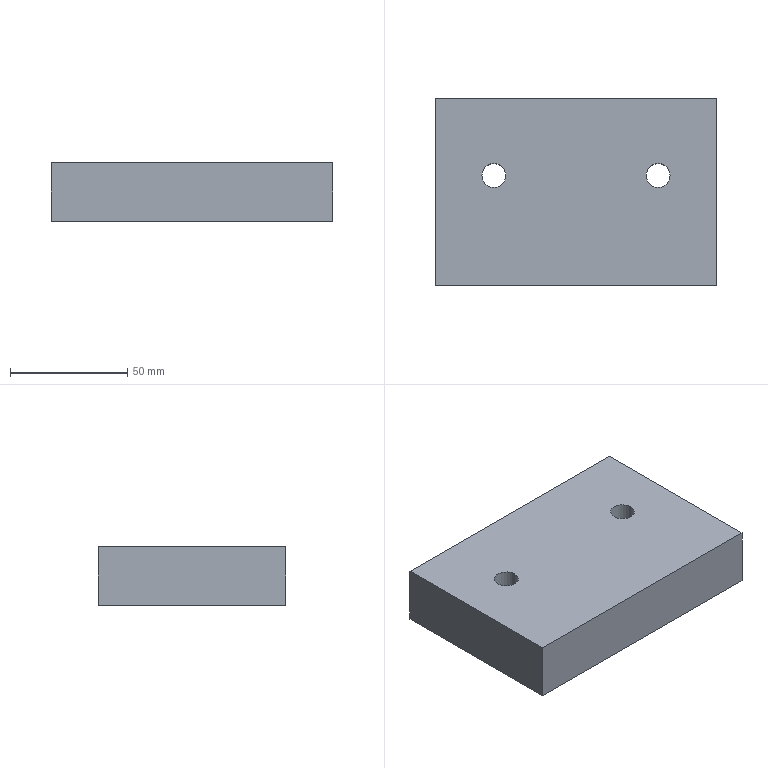Part | SolidWorks | features Extrusion 1, HoleWzd 1 | 1 solid | 10 faces | box 120 x 80 x 25 mm | volume 235914 mm3 | plane 6 | cylinder 4 | commonest cylinder face diameters 10.2 x4
STEP:
#1=CARTESIAN_POINT('',(-29.9,7.,0.));
#2=VERTEX_POINT('',#1);
#3=CARTESIAN_POINT('',(-40.1,7.,0.));
#4=VERTEX_POINT('',#3);
#5=CARTESIAN_POINT('',(-35.,7.,0.));
#6=DIRECTION('',(0.,0.,-1.));
#7=DIRECTION('',(-1.,0.,0.));
#8=AXIS2_PLACEMENT_3D('',#5,#6,#7);
#9=CIRCLE('',#8,5.1);
#10=EDGE_CURVE('',#2,#4,#9,.T.);
#11=ORIENTED_EDGE('',*,*,#10,.T.);
#12=CARTESIAN_POINT('',(-40.1,7.,25.));
#13=VERTEX_POINT('',#12);
#14=CARTESIAN_POINT('',(-40.1,7.,25.));
#15=DIRECTION('',(0.,0.,1.));
#16=VECTOR('',#15,1000.);
#17=LINE('',#14,#16);
#18=EDGE_CURVE('',#4,#13,#17,.T.);
#19=ORIENTED_EDGE('',*,*,#18,.T.);
#20=CARTESIAN_POINT('',(-29.9,7.,25.));
#21=VERTEX_POINT('',#20);
#22=CARTESIAN_POINT('',(-35.,7.,25.));
#23=DIRECTION('',(0.,0.,1.));
#24=DIRECTION('',(1.,0.,0.));
#25=AXIS2_PLACEMENT_3D('',#22,#23,#24);
#26=CIRCLE('',#25,5.1);
#27=EDGE_CURVE('',#13,#21,#26,.T.);
#28=ORIENTED_EDGE('',*,*,#27,.T.);
#29=CARTESIAN_POINT('',(-29.9,7.,25.));
#30=DIRECTION('',(0.,0.,1.));
#31=VECTOR('',#30,1000.);
#32=LINE('',#29,#31);
#33=EDGE_CURVE('',#2,#21,#32,.T.);
#34=ORIENTED_EDGE('',*,*,#33,.F.);
#35=EDGE_LOOP('',(#11,#19,#28,#34));
#36=FACE_OUTER_BOUND('',#35,.T.);
#37=CARTESIAN_POINT('',(-35.,7.,25.));
#38=DIRECTION('',(0.,0.,1.));
#39=DIRECTION('',(1.,0.,0.));
#40=AXIS2_PLACEMENT_3D('',#37,#38,#39);
#41=CYLINDRICAL_SURFACE('',#40,5.1);
#42=ADVANCED_FACE('',(#36),#41,.F.);
#43=CARTESIAN_POINT('',(40.1,7.,0.));
#44=VERTEX_POINT('',#43);
#45=CARTESIAN_POINT('',(29.9,7.,0.));
#46=VERTEX_POINT('',#45);
#47=CARTESIAN_POINT('',(35.,7.,0.));
#48=DIRECTION('',(0.,0.,-1.));
#49=DIRECTION('',(-1.,0.,0.));
#50=AXIS2_PLACEMENT_3D('',#47,#48,#49);
#51=CIRCLE('',#50,5.1);
#52=EDGE_CURVE('',#44,#46,#51,.T.);
#53=ORIENTED_EDGE('',*,*,#52,.T.);
#54=CARTESIAN_POINT('',(29.9,7.,25.));
#55=VERTEX_POINT('',#54);
#56=CARTESIAN_POINT('',(29.9,7.,25.));
#57=DIRECTION('',(0.,0.,1.));
#58=VECTOR('',#57,1000.);
#59=LINE('',#56,#58);
#60=EDGE_CURVE('',#46,#55,#59,.T.);
#61=ORIENTED_EDGE('',*,*,#60,.T.);
#62=CARTESIAN_POINT('',(40.1,7.,25.));
#63=VERTEX_POINT('',#62);
#64=CARTESIAN_POINT('',(35.,7.,25.));
#65=DIRECTION('',(0.,0.,1.));
#66=DIRECTION('',(1.,0.,0.));
#67=AXIS2_PLACEMENT_3D('',#64,#65,#66);
#68=CIRCLE('',#67,5.1);
#69=EDGE_CURVE('',#55,#63,#68,.T.);
#70=ORIENTED_EDGE('',*,*,#69,.T.);
#71=CARTESIAN_POINT('',(40.1,7.,25.));
#72=DIRECTION('',(0.,0.,1.));
#73=VECTOR('',#72,1000.);
#74=LINE('',#71,#73);
#75=EDGE_CURVE('',#44,#63,#74,.T.);
#76=ORIENTED_EDGE('',*,*,#75,.F.);
#77=EDGE_LOOP('',(#53,#61,#70,#76));
#78=FACE_OUTER_BOUND('',#77,.T.);
#79=CARTESIAN_POINT('',(35.,7.,25.));
#80=DIRECTION('',(0.,0.,1.));
#81=DIRECTION('',(1.,0.,0.));
#82=AXIS2_PLACEMENT_3D('',#79,#80,#81);
#83=CYLINDRICAL_SURFACE('',#82,5.1);
#84=ADVANCED_FACE('',(#78),#83,.F.);
#85=CARTESIAN_POINT('',(-60.,40.,0.));
#86=VERTEX_POINT('',#85);
#87=CARTESIAN_POINT('',(-60.,-40.,0.));
#88=VERTEX_POINT('',#87);
#89=CARTESIAN_POINT('',(-60.,40.,0.));
#90=DIRECTION('',(0.,-1.,0.));
#91=VECTOR('',#90,1000.);
#92=LINE('',#89,#91);
#93=EDGE_CURVE('',#86,#88,#92,.T.);
#94=ORIENTED_EDGE('',*,*,#93,.T.);
#95=CARTESIAN_POINT('',(-60.,-40.,25.));
#96=VERTEX_POINT('',#95);
#97=CARTESIAN_POINT('',(-60.,-40.,25.));
#98=DIRECTION('',(0.,0.,-1.));
#99=VECTOR('',#98,1000.);
#100=LINE('',#97,#99);
#101=EDGE_CURVE('',#96,#88,#100,.T.);
#102=ORIENTED_EDGE('',*,*,#101,.F.);
#103=CARTESIAN_POINT('',(-60.,40.,25.));
#104=VERTEX_POINT('',#103);
#105=CARTESIAN_POINT('',(-60.,40.,25.));
#106=DIRECTION('',(0.,-1.,0.));
#107=VECTOR('',#106,1000.);
#108=LINE('',#105,#107);
#109=EDGE_CURVE('',#104,#96,#108,.T.);
#110=ORIENTED_EDGE('',*,*,#109,.F.);
#111=CARTESIAN_POINT('',(-60.,40.,25.));
#112=DIRECTION('',(0.,0.,-1.));
#113=VECTOR('',#112,1000.);
#114=LINE('',#111,#113);
#115=EDGE_CURVE('',#104,#86,#114,.T.);
#116=ORIENTED_EDGE('',*,*,#115,.T.);
#117=EDGE_LOOP('',(#94,#102,#110,#116));
#118=FACE_OUTER_BOUND('',#117,.T.);
#119=CARTESIAN_POINT('',(-60.,40.,25.));
#120=DIRECTION('',(1.,0.,0.));
#121=DIRECTION('',(0.,1.,0.));
#122=AXIS2_PLACEMENT_3D('',#119,#120,#121);
#123=PLANE('',#122);
#124=ADVANCED_FACE('',(#118),#123,.F.);
#125=CARTESIAN_POINT('',(60.,-40.,0.));
#126=VERTEX_POINT('',#125);
#127=CARTESIAN_POINT('',(60.,-40.,0.));
#128=DIRECTION('',(1.,0.,0.));
#129=VECTOR('',#128,1000.);
#130=LINE('',#127,#129);
#131=EDGE_CURVE('',#88,#126,#130,.T.);
#132=ORIENTED_EDGE('',*,*,#131,.T.);
#133=CARTESIAN_POINT('',(60.,-40.,25.));
#134=VERTEX_POINT('',#133);
#135=CARTESIAN_POINT('',(60.,-40.,25.));
#136=DIRECTION('',(0.,0.,-1.));
#137=VECTOR('',#136,1000.);
#138=LINE('',#135,#137);
#139=EDGE_CURVE('',#134,#126,#138,.T.);
#140=ORIENTED_EDGE('',*,*,#139,.F.);
#141=CARTESIAN_POINT('',(60.,-40.,25.));
#142=DIRECTION('',(1.,0.,0.));
#143=VECTOR('',#142,1000.);
#144=LINE('',#141,#143);
#145=EDGE_CURVE('',#96,#134,#144,.T.);
#146=ORIENTED_EDGE('',*,*,#145,.F.);
#147=ORIENTED_EDGE('',*,*,#101,.T.);
#148=EDGE_LOOP('',(#132,#140,#146,#147));
#149=FACE_OUTER_BOUND('',#148,.T.);
#150=CARTESIAN_POINT('',(60.,-40.,25.));
#151=DIRECTION('',(0.,1.,0.));
#152=DIRECTION('',(-1.,0.,0.));
#153=AXIS2_PLACEMENT_3D('',#150,#151,#152);
#154=PLANE('',#153);
#155=ADVANCED_FACE('',(#149),#154,.F.);
#156=CARTESIAN_POINT('',(60.,40.,0.));
#157=VERTEX_POINT('',#156);
#158=CARTESIAN_POINT('',(60.,40.,0.));
#159=DIRECTION('',(0.,1.,0.));
#160=VECTOR('',#159,1000.);
#161=LINE('',#158,#160);
#162=EDGE_CURVE('',#126,#157,#161,.T.);
#163=ORIENTED_EDGE('',*,*,#162,.T.);
#164=CARTESIAN_POINT('',(60.,40.,25.));
#165=VERTEX_POINT('',#164);
#166=CARTESIAN_POINT('',(60.,40.,25.));
#167=DIRECTION('',(0.,0.,-1.));
#168=VECTOR('',#167,1000.);
#169=LINE('',#166,#168);
#170=EDGE_CURVE('',#165,#157,#169,.T.);
#171=ORIENTED_EDGE('',*,*,#170,.F.);
#172=CARTESIAN_POINT('',(60.,40.,25.));
#173=DIRECTION('',(0.,1.,0.));
#174=VECTOR('',#173,1000.);
#175=LINE('',#172,#174);
#176=EDGE_CURVE('',#134,#165,#175,.T.);
#177=ORIENTED_EDGE('',*,*,#176,.F.);
#178=ORIENTED_EDGE('',*,*,#139,.T.);
#179=EDGE_LOOP('',(#163,#171,#177,#178));
#180=FACE_OUTER_BOUND('',#179,.T.);
#181=CARTESIAN_POINT('',(60.,40.,25.));
#182=DIRECTION('',(-1.,0.,0.));
#183=DIRECTION('',(0.,-1.,0.));
#184=AXIS2_PLACEMENT_3D('',#181,#182,#183);
#185=PLANE('',#184);
#186=ADVANCED_FACE('',(#180),#185,.F.);
#187=CARTESIAN_POINT('',(60.,40.,0.));
#188=DIRECTION('',(-1.,0.,0.));
#189=VECTOR('',#188,1000.);
#190=LINE('',#187,#189);
#191=EDGE_CURVE('',#157,#86,#190,.T.);
#192=ORIENTED_EDGE('',*,*,#191,.T.);
#193=ORIENTED_EDGE('',*,*,#115,.F.);
#194=CARTESIAN_POINT('',(60.,40.,25.));
#195=DIRECTION('',(-1.,0.,0.));
#196=VECTOR('',#195,1000.);
#197=LINE('',#194,#196);
#198=EDGE_CURVE('',#165,#104,#197,.T.);
#199=ORIENTED_EDGE('',*,*,#198,.F.);
#200=ORIENTED_EDGE('',*,*,#170,.T.);
#201=EDGE_LOOP('',(#192,#193,#199,#200));
#202=FACE_OUTER_BOUND('',#201,.T.);
#203=CARTESIAN_POINT('',(60.,40.,25.));
#204=DIRECTION('',(0.,-1.,0.));
#205=DIRECTION('',(1.,0.,0.));
#206=AXIS2_PLACEMENT_3D('',#203,#204,#205);
#207=PLANE('',#206);
#208=ADVANCED_FACE('',(#202),#207,.F.);
#209=CARTESIAN_POINT('',(-35.,7.,25.));
#210=DIRECTION('',(0.,0.,1.));
#211=DIRECTION('',(1.,0.,0.));
#212=AXIS2_PLACEMENT_3D('',#209,#210,#211);
#213=CIRCLE('',#212,5.1);
#214=EDGE_CURVE('',#21,#13,#213,.T.);
#215=ORIENTED_EDGE('',*,*,#214,.F.);
#216=ORIENTED_EDGE('',*,*,#27,.F.);
#217=EDGE_LOOP('',(#215,#216));
#218=FACE_BOUND('',#217,.T.);
#219=CARTESIAN_POINT('',(35.,7.,25.));
#220=DIRECTION('',(0.,0.,1.));
#221=DIRECTION('',(1.,0.,0.));
#222=AXIS2_PLACEMENT_3D('',#219,#220,#221);
#223=CIRCLE('',#222,5.1);
#224=EDGE_CURVE('',#63,#55,#223,.T.);
#225=ORIENTED_EDGE('',*,*,#224,.F.);
#226=ORIENTED_EDGE('',*,*,#69,.F.);
#227=EDGE_LOOP('',(#225,#226));
#228=FACE_BOUND('',#227,.T.);
#229=ORIENTED_EDGE('',*,*,#109,.T.);
#230=ORIENTED_EDGE('',*,*,#145,.T.);
#231=ORIENTED_EDGE('',*,*,#176,.T.);
#232=ORIENTED_EDGE('',*,*,#198,.T.);
#233=EDGE_LOOP('',(#229,#230,#231,#232));
#234=FACE_OUTER_BOUND('',#233,.T.);
#235=CARTESIAN_POINT('',(0.,0.,25.));
#236=DIRECTION('',(0.,0.,-1.));
#237=DIRECTION('',(-1.,0.,0.));
#238=AXIS2_PLACEMENT_3D('',#235,#236,#237);
#239=PLANE('',#238);
#240=ADVANCED_FACE('',(#218,#228,#234),#239,.F.);
#241=ORIENTED_EDGE('',*,*,#10,.F.);
#242=CARTESIAN_POINT('',(-35.,7.,0.));
#243=DIRECTION('',(0.,0.,-1.));
#244=DIRECTION('',(-1.,0.,0.));
#245=AXIS2_PLACEMENT_3D('',#242,#243,#244);
#246=CIRCLE('',#245,5.1);
#247=EDGE_CURVE('',#4,#2,#246,.T.);
#248=ORIENTED_EDGE('',*,*,#247,.F.);
#249=EDGE_LOOP('',(#241,#248));
#250=FACE_BOUND('',#249,.T.);
#251=ORIENTED_EDGE('',*,*,#52,.F.);
#252=CARTESIAN_POINT('',(35.,7.,0.));
#253=DIRECTION('',(0.,0.,-1.));
#254=DIRECTION('',(-1.,0.,0.));
#255=AXIS2_PLACEMENT_3D('',#252,#253,#254);
#256=CIRCLE('',#255,5.1);
#257=EDGE_CURVE('',#46,#44,#256,.T.);
#258=ORIENTED_EDGE('',*,*,#257,.F.);
#259=EDGE_LOOP('',(#251,#258));
#260=FACE_BOUND('',#259,.T.);
#261=ORIENTED_EDGE('',*,*,#93,.F.);
#262=ORIENTED_EDGE('',*,*,#191,.F.);
#263=ORIENTED_EDGE('',*,*,#162,.F.);
#264=ORIENTED_EDGE('',*,*,#131,.F.);
#265=EDGE_LOOP('',(#261,#262,#263,#264));
#266=FACE_OUTER_BOUND('',#265,.T.);
#267=CARTESIAN_POINT('',(0.,0.,0.));
#268=DIRECTION('',(0.,0.,-1.));
#269=DIRECTION('',(-1.,0.,0.));
#270=AXIS2_PLACEMENT_3D('',#267,#268,#269);
#271=PLANE('',#270);
#272=ADVANCED_FACE('',(#250,#260,#266),#271,.T.);
#273=ORIENTED_EDGE('',*,*,#60,.F.);
#274=ORIENTED_EDGE('',*,*,#257,.T.);
#275=ORIENTED_EDGE('',*,*,#75,.T.);
#276=ORIENTED_EDGE('',*,*,#224,.T.);
#277=EDGE_LOOP('',(#273,#274,#275,#276));
#278=FACE_OUTER_BOUND('',#277,.T.);
#279=CARTESIAN_POINT('',(35.,7.,25.));
#280=DIRECTION('',(0.,0.,1.));
#281=DIRECTION('',(1.,0.,0.));
#282=AXIS2_PLACEMENT_3D('',#279,#280,#281);
#283=CYLINDRICAL_SURFACE('',#282,5.1);
#284=ADVANCED_FACE('',(#278),#283,.F.);
#285=ORIENTED_EDGE('',*,*,#18,.F.);
#286=ORIENTED_EDGE('',*,*,#247,.T.);
#287=ORIENTED_EDGE('',*,*,#33,.T.);
#288=ORIENTED_EDGE('',*,*,#214,.T.);
#289=EDGE_LOOP('',(#285,#286,#287,#288));
#290=FACE_OUTER_BOUND('',#289,.T.);
#291=CARTESIAN_POINT('',(-35.,7.,25.));
#292=DIRECTION('',(0.,0.,1.));
#293=DIRECTION('',(1.,0.,0.));
#294=AXIS2_PLACEMENT_3D('',#291,#292,#293);
#295=CYLINDRICAL_SURFACE('',#294,5.1);
#296=ADVANCED_FACE('',(#290),#295,.F.);
#297=CLOSED_SHELL('',(#42,#84,#124,#155,#186,#208,#240,#272,#284,#296));
#298=MANIFOLD_SOLID_BREP('',#297);
#299=CARTESIAN_POINT('',(0.,0.,0.));
#300=DIRECTION('',(0.,0.,1.));
#301=DIRECTION('',(1.,0.,0.));
#302=AXIS2_PLACEMENT_3D('',#299,#300,#301);
#303=(LENGTH_UNIT()NAMED_UNIT(*)SI_UNIT(.MILLI.,.METRE.));
#304=UNCERTAINTY_MEASURE_WITH_UNIT(LENGTH_MEASURE(0.00001),#303,'','');
#305=(NAMED_UNIT(*)PLANE_ANGLE_UNIT()SI_UNIT($,.RADIAN.));
#306=(NAMED_UNIT(*)SI_UNIT($,.STERADIAN.)SOLID_ANGLE_UNIT());
#307=(GEOMETRIC_REPRESENTATION_CONTEXT(3)GLOBAL_UNCERTAINTY_ASSIGNED_CONTEXT((#304))GLOBAL_UNIT_ASSIGNED_CONTEXT((#303,#305,#306))REPRESENTATION_CONTEXT('',''));
#308=ADVANCED_BREP_SHAPE_REPRESENTATION('',(#298,#302),#307);